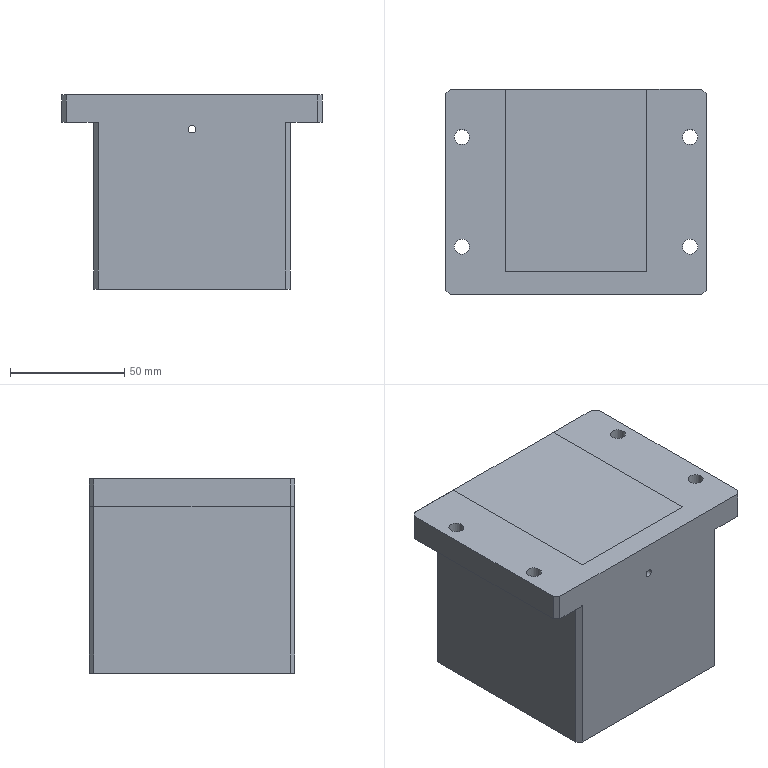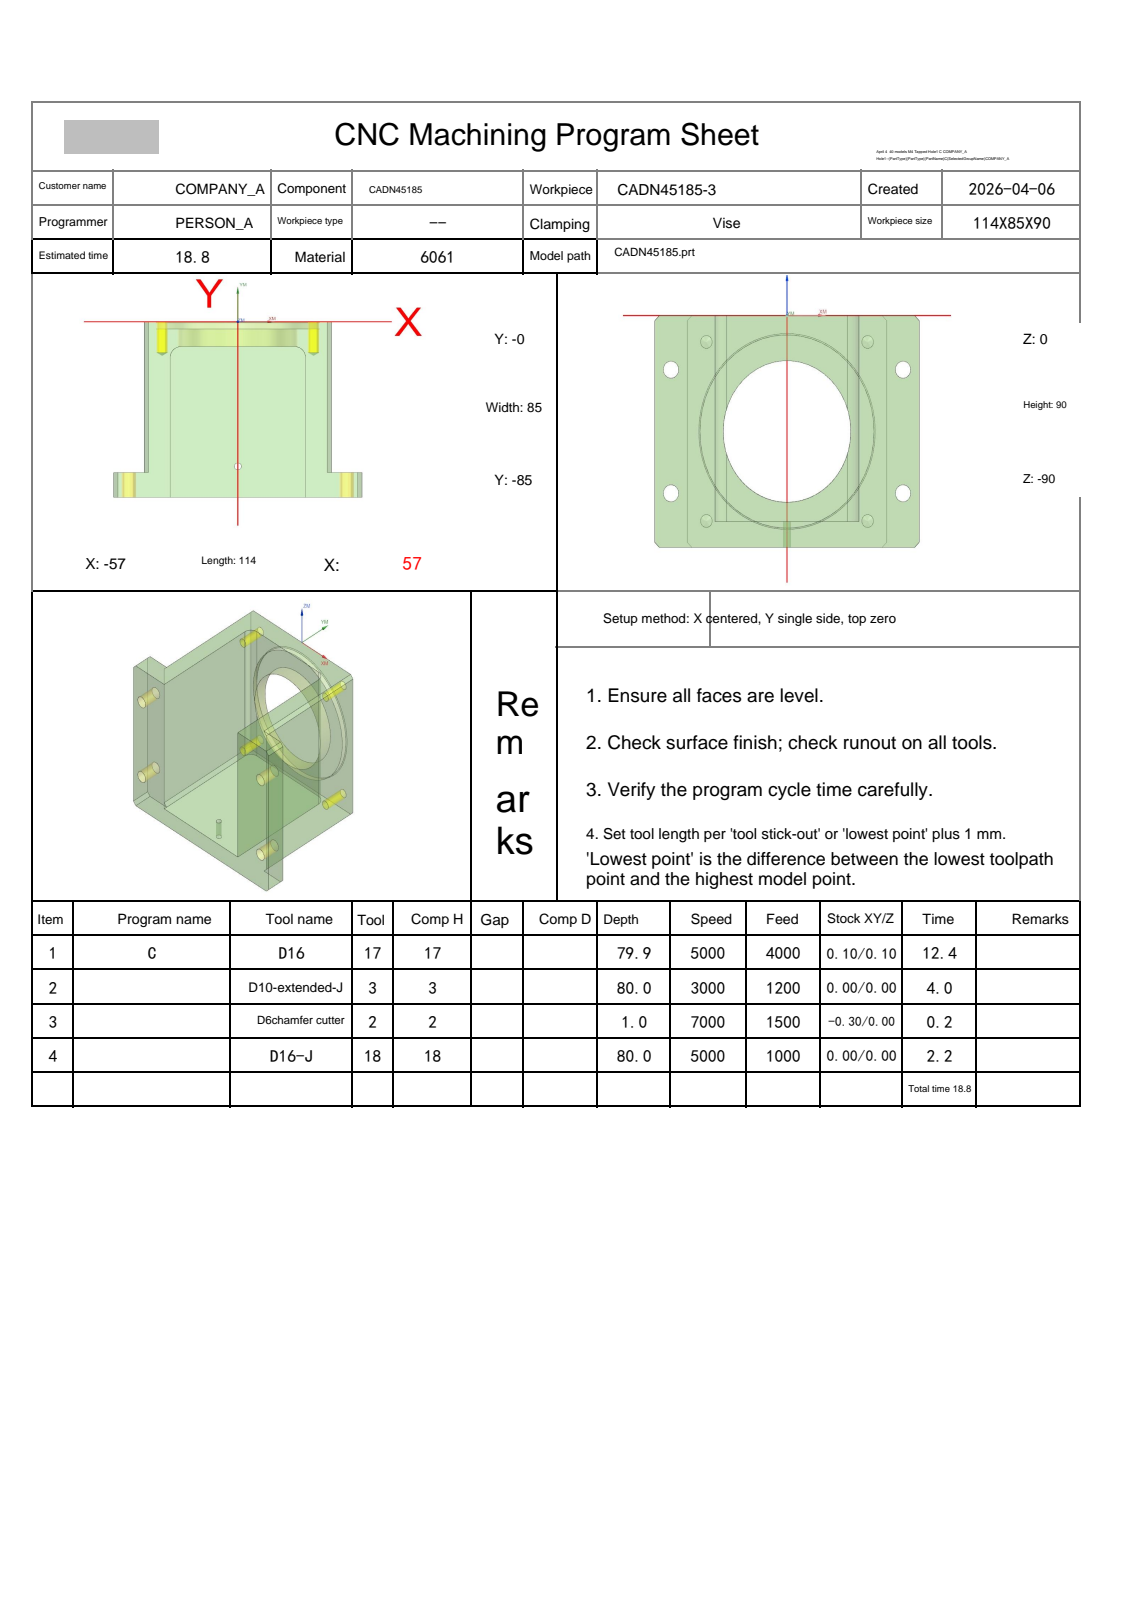NC program | NX | posted by the shop | part box 114 x 90 x 85 mm
Lines 2624 to 3642 of 14367:
N2 T03 M06
(D10-extended-J  D=10. R=0. H=03 ce=0.00 di=0.00)
G00 G90 G54 X24.999 Y-21.95 M03 S3000
G43 H03 Z50.
M08
Z.5
G01 X25.012 Y-21.947 Z.348 F1200.
X25.048 Y-21.938 Z.211
X25.103 Y-21.922 Z.089
X25.175 Y-21.899 Z-.02
X25.258 Y-21.868 Z-.115
X25.351 Y-21.828 Z-.198
X25.449 Y-21.778 Z-.269
X25.549 Y-21.718 Z-.329
X25.648 Y-21.647 Z-.378
X25.74 Y-21.564 Z-.419
X25.824 Y-21.469 Z-.45
X25.896 Y-21.361 Z-.473
X25.951 Y-21.238 Z-.488
X25.987 Y-21.102 Z-.497
X26. Y-20.95 Z-.5
Y-17.
X22.05
X21.955 Y-17.015 Z-.501
X21.88 Y-17.057 Z-.503
X21.826 Y-17.126 Z-.507
X21.791 Y-17.216 Z-.512
X21.774 Y-17.328 Z-.518
X21.775 Y-17.456 Z-.525
X21.79 Y-17.6 Z-.534
X21.821 Y-17.757 Z-.543
X21.864 Y-17.924 Z-.554
X21.92 Y-18.098 Z-.566
X21.987 Y-18.278 Z-.578
X22.064 Y-18.46 Z-.591
X22.15 Y-18.641 Z-.605
X22.243 Y-18.821 Z-.62
X22.485 Y-19.219 Z-.656
X22.761 Y-19.589 Z-.695
X23.07 Y-19.929 Z-.735
X23.41 Y-20.237 Z-.775
X23.78 Y-20.513 Z-.816
X24.179 Y-20.755 Z-.856
X24.358 Y-20.849 Z-.872
X24.54 Y-20.934 Z-.888
X24.722 Y-21.011 Z-.904
X24.901 Y-21.078 Z-.918
X25.076 Y-21.135 Z-.932
X25.243 Y-21.178 Z-.945
X25.399 Y-21.209 Z-.957
X25.543 Y-21.225 Z-.968
X25.672 Z-.977
X25.784 Y-21.209 Z-.985
X25.874 Y-21.174 Z-.991
X25.942 Y-21.12 Z-.996
X25.985 Y-21.045 Z-.999
X26. Y-20.95 Z-1.
Y-17.
X22.051
X21.955 Y-17.015 Z-1.001
X21.88 Y-17.057 Z-1.003
X21.826 Y-17.126 Z-1.007
X21.791 Y-17.216 Z-1.012
X21.774 Y-17.328 Z-1.018
Y-17.456 Z-1.025
X21.79 Y-17.6 Z-1.034
X21.82 Y-17.757 Z-1.044
X21.863 Y-17.924 Z-1.054
X21.919 Y-18.098 Z-1.066
X21.986 Y-18.278 Z-1.078
X22.063 Y-18.46 Z-1.091
X22.148 Y-18.641 Z-1.105
X22.241 Y-18.821 Z-1.12
X22.483 Y-19.219 Z-1.156
X22.759 Y-19.589 Z-1.195
X23.068 Y-19.929 Z-1.235
X23.408 Y-20.237 Z-1.276
X23.778 Y-20.513 Z-1.316
X24.178 Y-20.755 Z-1.356
X24.357 Y-20.849 Z-1.372
X24.539 Y-20.934 Z-1.388
X24.721 Y-21.011 Z-1.404
X24.901 Y-21.078 Z-1.418
X25.075 Y-21.135 Z-1.432
X25.242 Y-21.178 Z-1.445
X25.399 Y-21.209 Z-1.457
X25.543 Y-21.225 Z-1.468
X25.672 Z-1.477
X25.783 Y-21.209 Z-1.485
X25.874 Y-21.174 Z-1.491
X25.942 Y-21.12 Z-1.496
X25.985 Y-21.045 Z-1.499
X26. Y-20.95 Z-1.5
Y-17.
X22.051
X21.954 Y-17.015 Z-1.501
X21.88 Y-17.057 Z-1.503
X21.826 Y-17.126 Z-1.507
X21.791 Y-17.216 Z-1.512
X21.774 Y-17.328 Z-1.518
X21.773 Y-17.456 Z-1.525
X21.789 Y-17.6 Z-1.534
X21.819 Y-17.757 Z-1.544
X21.862 Y-17.924 Z-1.554
X21.918 Y-18.098 Z-1.566
X21.985 Y-18.278 Z-1.578
X22.061 Y-18.46 Z-1.592
X22.146 Y-18.641 Z-1.606
X22.239 Y-18.821 Z-1.62
X22.482 Y-19.22 Z-1.656
X22.758 Y-19.589 Z-1.695
X23.066 Y-19.929 Z-1.735
X23.406 Y-20.237 Z-1.776
X23.777 Y-20.513 Z-1.816
X24.177 Y-20.755 Z-1.856
X24.356 Y-20.849 Z-1.872
X24.538 Y-20.934 Z-1.888
X24.721 Y-21.011 Z-1.904
X24.9 Y-21.078 Z-1.918
X25.075 Y-21.135 Z-1.932
X25.242 Y-21.178 Z-1.945
X25.399 Y-21.209 Z-1.957
X25.543 Y-21.225 Z-1.968
X25.672 Z-1.977
X25.783 Y-21.209 Z-1.985
X25.874 Y-21.174 Z-1.991
X25.942 Y-21.12 Z-1.996
X25.985 Y-21.045 Z-1.999
X26. Y-20.95 Z-2.
Y-17.
X22.05
X21.954 Y-17.015 Z-2.001
X21.88 Y-17.057 Z-2.003
X21.826 Y-17.126 Z-2.007
X21.79 Y-17.216 Z-2.012
X21.773 Y-17.328 Z-2.018
Y-17.456 Z-2.025
X21.788 Y-17.601 Z-2.034
X21.818 Y-17.757 Z-2.044
X21.861 Y-17.924 Z-2.054
X21.917 Y-18.098 Z-2.066
X21.983 Y-18.278 Z-2.079
X22.059 Y-18.46 Z-2.092
X22.145 Y-18.641 Z-2.106
X22.238 Y-18.821 Z-2.12
X22.48 Y-19.22 Z-2.157
X22.756 Y-19.589 Z-2.195
X23.064 Y-19.929 Z-2.235
X23.405 Y-20.237 Z-2.276
X23.776 Y-20.513 Z-2.317
X24.176 Y-20.755 Z-2.356
X24.355 Y-20.849 Z-2.373
X24.538 Y-20.934 Z-2.388
X24.72 Y-21.011 Z-2.404
X24.9 Y-21.078 Z-2.419
X25.074 Y-21.135 Z-2.432
X25.241 Y-21.178 Z-2.445
X25.398 Y-21.209 Z-2.457
X25.543 Y-21.225 Z-2.468
X25.672 Z-2.477
X25.783 Y-21.209 Z-2.485
X25.874 Y-21.174 Z-2.491
X25.942 Y-21.12 Z-2.496
X25.985 Y-21.045 Z-2.499
X26. Y-20.95 Z-2.5
Y-17.
X22.05
X21.954 Y-17.015 Z-2.501
X21.88 Y-17.057 Z-2.503
X21.825 Y-17.126 Z-2.507
X21.79 Y-17.216 Z-2.512
X21.773 Y-17.328 Z-2.518
X21.772 Y-17.456 Z-2.526
X21.787 Y-17.601 Z-2.534
X21.817 Y-17.757 Z-2.544
X21.86 Y-17.924 Z-2.555
X21.915 Y-18.098 Z-2.566
X21.982 Y-18.278 Z-2.579
X22.058 Y-18.46 Z-2.592
X22.143 Y-18.641 Z-2.606
X22.236 Y-18.821 Z-2.621
X22.478 Y-19.22 Z-2.657
X22.754 Y-19.589 Z-2.695
X23.063 Y-19.929 Z-2.736
X23.403 Y-20.237 Z-2.776
X23.774 Y-20.513 Z-2.817
X24.175 Y-20.755 Z-2.856
X24.354 Y-20.849 Z-2.873
X24.537 Y-20.934 Z-2.889
X24.719 Y-21.011 Z-2.904
X24.899 Y-21.078 Z-2.919
X25.074 Y-21.135 Z-2.932
X25.241 Y-21.178 Z-2.945
X25.398 Y-21.209 Z-2.957
X25.543 Y-21.225 Z-2.968
X25.672 Z-2.977
X25.783 Y-21.209 Z-2.985
X25.874 Y-21.174 Z-2.991
X25.942 Y-21.12 Z-2.996
X25.985 Y-21.045 Z-2.999
X26. Y-20.95 Z-3.
Y-17.
X22.051
X21.954 Y-17.015 Z-3.001
X21.88 Y-17.057 Z-3.003
X21.825 Y-17.126 Z-3.007
X21.79 Y-17.216 Z-3.012
X21.772 Y-17.328 Z-3.018
Y-17.456 Z-3.026
X21.787 Y-17.601 Z-3.034
X21.816 Y-17.757 Z-3.044
X21.859 Y-17.924 Z-3.055
X21.914 Y-18.098 Z-3.066
X21.98 Y-18.278 Z-3.079
X22.056 Y-18.46 Z-3.092
X22.141 Y-18.642 Z-3.106
X22.234 Y-18.821 Z-3.121
X22.476 Y-19.22 Z-3.157
X22.752 Y-19.589 Z-3.196
X23.061 Y-19.929 Z-3.236
X23.402 Y-20.237 Z-3.276
X23.773 Y-20.513 Z-3.317
X24.174 Y-20.755 Z-3.356
X24.353 Y-20.849 Z-3.373
X24.536 Y-20.934 Z-3.389
X24.718 Y-21.011 Z-3.404
X24.898 Y-21.078 Z-3.419
X25.073 Y-21.135 Z-3.432
X25.241 Y-21.178 Z-3.445
X25.398 Y-21.209 Z-3.457
X25.542 Y-21.225 Z-3.468
X25.672 Z-3.477
X25.783 Y-21.209 Z-3.485
X25.874 Y-21.174 Z-3.491
X25.942 Y-21.12 Z-3.496
X25.985 Y-21.045 Z-3.499
X26. Y-20.95 Z-3.5
Y-17.
X22.05
X21.954 Y-17.015 Z-3.501
X21.88 Y-17.058 Z-3.503
X21.825 Y-17.126 Z-3.507
X21.789 Y-17.216 Z-3.512
X21.772 Y-17.328 Z-3.518
X21.771 Y-17.456 Z-3.526
X21.786 Y-17.601 Z-3.534
X21.815 Y-17.757 Z-3.544
X21.858 Y-17.924 Z-3.555
X21.913 Y-18.098 Z-3.567
X21.979 Y-18.278 Z-3.579
X22.055 Y-18.46 Z-3.592
X22.139 Y-18.642 Z-3.606
X22.232 Y-18.821 Z-3.621
X22.474 Y-19.22 Z-3.657
X22.75 Y-19.589 Z-3.696
X23.059 Y-19.929 Z-3.736
X23.4 Y-20.237 Z-3.777
X23.772 Y-20.513 Z-3.817
X24.173 Y-20.755 Z-3.856
X24.353 Y-20.849 Z-3.873
X24.535 Y-20.934 Z-3.889
X24.718 Y-21.011 Z-3.904
X24.898 Y-21.078 Z-3.919
X25.073 Y-21.135 Z-3.933
X25.24 Y-21.178 Z-3.945
X25.398 Y-21.209 Z-3.957
X25.542 Y-21.225 Z-3.968
X25.671 Z-3.977
X25.783 Y-21.209 Z-3.985
X25.874 Y-21.174 Z-3.991
X25.942 Y-21.12 Z-3.996
X25.985 Y-21.045 Z-3.999
X26. Y-20.95 Z-4.
Y-17.
X22.05
X21.954 Y-17.015 Z-4.001
X21.88 Y-17.058 Z-4.003
X21.825 Y-17.126 Z-4.007
X21.789 Y-17.216 Z-4.012
X21.771 Y-17.328 Z-4.018
X21.77 Y-17.456 Z-4.026
X21.785 Y-17.601 Z-4.034
X21.814 Y-17.757 Z-4.044
X21.857 Y-17.924 Z-4.055
X21.911 Y-18.098 Z-4.067
X21.977 Y-18.278 Z-4.079
X22.053 Y-18.46 Z-4.093
X22.138 Y-18.642 Z-4.107
X22.23 Y-18.821 Z-4.121
X22.472 Y-19.22 Z-4.158
X22.748 Y-19.589 Z-4.196
X23.057 Y-19.929 Z-4.236
X23.399 Y-20.237 Z-4.277
X23.77 Y-20.513 Z-4.317
X24.172 Y-20.755 Z-4.357
X24.352 Y-20.849 Z-4.373
X24.534 Y-20.934 Z-4.389
X24.717 Y-21.011 Z-4.404
X24.897 Y-21.078 Z-4.419
X25.072 Y-21.135 Z-4.433
X25.24 Y-21.178 Z-4.445
X25.397 Y-21.209 Z-4.457
X25.542 Y-21.225 Z-4.468
X25.671 Z-4.477
X25.783 Y-21.209 Z-4.485
X25.874 Y-21.174 Z-4.491
X25.942 Y-21.12 Z-4.496
X25.985 Y-21.045 Z-4.499
X26. Y-20.95 Z-4.5
Y-17.
X22.051
X21.954 Y-17.015 Z-4.501
X21.879 Y-17.058 Z-4.503
X21.825 Y-17.126 Z-4.507
X21.789 Y-17.216 Z-4.512
X21.771 Y-17.328 Z-4.518
X21.77 Y-17.456 Z-4.526
X21.784 Y-17.601 Z-4.535
X21.813 Y-17.757 Z-4.544
X21.855 Y-17.924 Z-4.555
X21.91 Y-18.099 Z-4.567
X21.976 Y-18.278 Z-4.579
X22.051 Y-18.46 Z-4.593
X22.136 Y-18.642 Z-4.607
X22.228 Y-18.821 Z-4.621
X22.47 Y-19.22 Z-4.658
X22.746 Y-19.589 Z-4.696
X23.055 Y-19.929 Z-4.736
X23.397 Y-20.237 Z-4.777
X23.769 Y-20.513 Z-4.817
X24.17 Y-20.756 Z-4.857
X24.351 Y-20.849 Z-4.873
X24.534 Y-20.934 Z-4.889
X24.716 Y-21.011 Z-4.904
X24.897 Y-21.078 Z-4.919
X25.072 Y-21.135 Z-4.933
X25.239 Y-21.178 Z-4.945
X25.397 Y-21.209 Z-4.957
X25.542 Y-21.225 Z-4.968
X25.671 Z-4.977
X25.783 Y-21.209 Z-4.985
X25.874 Y-21.174 Z-4.991
X25.942 Y-21.12 Z-4.996
X25.985 Y-21.045 Z-4.999
X26. Y-20.95 Z-5.
Y-17.
X22.05
X21.954 Y-17.015 Z-5.001
X21.879 Y-17.058 Z-5.003
X21.824 Y-17.126 Z-5.007
X21.789 Y-17.216 Z-5.012
X21.771 Y-17.328 Z-5.018
X21.769 Y-17.457 Z-5.026
X21.783 Y-17.601 Z-5.035
X21.812 Y-17.757 Z-5.044
X21.854 Y-17.924 Z-5.055
X21.909 Y-18.099 Z-5.067
X21.974 Y-18.278 Z-5.08
X22.05 Y-18.46 Z-5.093
X22.134 Y-18.642 Z-5.107
X22.227 Y-18.821 Z-5.122
X22.468 Y-19.22 Z-5.158
X22.744 Y-19.59 Z-5.197
X23.054 Y-19.929 Z-5.237
X23.395 Y-20.237 Z-5.277
X23.768 Y-20.513 Z-5.317
X24.169 Y-20.756 Z-5.357
X24.35 Y-20.849 Z-5.373
X24.533 Y-20.934 Z-5.389
X24.716 Y-21.011 Z-5.404
X24.896 Y-21.079 Z-5.419
X25.071 Y-21.135 Z-5.433
X25.239 Y-21.178 Z-5.446
X25.397 Y-21.209 Z-5.457
X25.541 Y-21.225 Z-5.468
X25.671 Z-5.477
X25.783 Y-21.209 Z-5.485
X25.874 Y-21.174 Z-5.491
X25.942 Y-21.12 Z-5.496
X25.985 Y-21.045 Z-5.499
X26. Y-20.95 Z-5.5
Y-17.
X22.05
X21.954 Y-17.015 Z-5.501
X21.879 Y-17.058 Z-5.503
X21.824 Y-17.126 Z-5.507
X21.788 Y-17.216 Z-5.512
X21.77 Y-17.328 Z-5.518
X21.769 Y-17.457 Z-5.526
X21.783 Y-17.601 Z-5.535
X21.811 Y-17.757 Z-5.545
X21.853 Y-17.924 Z-5.555
X21.907 Y-18.099 Z-5.567
X21.973 Y-18.278 Z-5.58
X22.048 Y-18.46 Z-5.593
X22.133 Y-18.642 Z-5.607
X22.225 Y-18.821 Z-5.622
X22.466 Y-19.22 Z-5.658
X22.742 Y-19.59 Z-5.697
X23.052 Y-19.929 Z-5.737
X23.394 Y-20.237 Z-5.777
X23.766 Y-20.513 Z-5.818
X24.168 Y-20.756 Z-5.857
X24.349 Y-20.849 Z-5.873
X24.532 Y-20.934 Z-5.889
X24.715 Y-21.011 Z-5.904
X24.895 Y-21.079 Z-5.919
X25.071 Y-21.135 Z-5.933
X25.239 Y-21.178 Z-5.946
X25.396 Y-21.209 Z-5.957
X25.541 Y-21.225 Z-5.968
X25.671 Z-5.977
X25.782 Y-21.209 Z-5.985
X25.874 Y-21.174 Z-5.991
X25.942 Y-21.12 Z-5.996
X25.985 Y-21.045 Z-5.999
X26. Y-20.95 Z-6.
Y-17.
X22.051
X21.954 Y-17.015 Z-6.001
X21.879 Y-17.058 Z-6.003
X21.824 Y-17.126 Z-6.007
X21.788 Y-17.216 Z-6.012
X21.77 Y-17.328 Z-6.018
X21.768 Y-17.457 Z-6.026
X21.782 Y-17.601 Z-6.035
X21.81 Y-17.757 Z-6.045
X21.852 Y-17.924 Z-6.056
X21.906 Y-18.099 Z-6.067
X21.971 Y-18.278 Z-6.08
X22.047 Y-18.46 Z-6.093
X22.131 Y-18.642 Z-6.107
X22.223 Y-18.821 Z-6.122
X22.464 Y-19.22 Z-6.158
X22.74 Y-19.59 Z-6.197
X23.05 Y-19.929 Z-6.237
X23.392 Y-20.237 Z-6.277
X23.765 Y-20.513 Z-6.318
X24.167 Y-20.756 Z-6.357
X24.348 Y-20.849 Z-6.373
X24.531 Y-20.934 Z-6.389
X24.714 Y-21.011 Z-6.404
X24.895 Y-21.079 Z-6.419
X25.07 Y-21.135 Z-6.433
X25.238 Y-21.178 Z-6.446
X25.396 Y-21.209 Z-6.457
X25.541 Y-21.225 Z-6.468
X25.671 Z-6.477
X25.782 Y-21.209 Z-6.485
X25.874 Y-21.174 Z-6.491
X25.942 Y-21.12 Z-6.496
X25.985 Y-21.045 Z-6.499
X26. Y-20.95 Z-6.5
Y-17.
X22.05
X21.954 Y-17.015 Z-6.501
X21.879 Y-17.058 Z-6.503
X21.824 Y-17.126 Z-6.507
X21.788 Y-17.216 Z-6.512
X21.769 Y-17.328 Z-6.518
X21.767 Y-17.457 Z-6.526
X21.781 Y-17.601 Z-6.535
X21.809 Y-17.757 Z-6.545
X21.851 Y-17.924 Z-6.556
X21.905 Y-18.099 Z-6.567
X21.97 Y-18.278 Z-6.58
X22.045 Y-18.46 Z-6.593
X22.129 Y-18.642 Z-6.608
X22.221 Y-18.821 Z-6.622
X22.462 Y-19.22 Z-6.659
X22.738 Y-19.59 Z-6.697
X23.048 Y-19.929 Z-6.737
X23.391 Y-20.237 Z-6.778
X23.764 Y-20.513 Z-6.818
X24.166 Y-20.756 Z-6.857
X24.347 Y-20.849 Z-6.873
X24.53 Y-20.934 Z-6.889
X24.714 Y-21.011 Z-6.905
X24.894 Y-21.079 Z-6.919
X25.07 Y-21.135 Z-6.933
X25.238 Y-21.179 Z-6.946
X25.396 Y-21.209 Z-6.957
X25.541 Y-21.225 Z-6.968
X25.67 Z-6.977
X25.782 Y-21.209 Z-6.985
X25.874 Y-21.174 Z-6.991
X25.942 Y-21.12 Z-6.996
X25.985 Y-21.045 Z-6.999
X26. Y-20.95 Z-7.
Y-17.
X22.051
X21.954 Y-17.015 Z-7.001
X21.879 Y-17.058 Z-7.003
X21.824 Y-17.126 Z-7.007
X21.787 Y-17.216 Z-7.012
X21.769 Y-17.328 Z-7.018
X21.767 Y-17.457 Z-7.026
X21.78 Y-17.601 Z-7.035
X21.808 Y-17.757 Z-7.045
X21.85 Y-17.924 Z-7.056
X21.904 Y-18.099 Z-7.068
X21.968 Y-18.278 Z-7.08
X22.043 Y-18.46 Z-7.094
X22.127 Y-18.642 Z-7.108
X22.219 Y-18.821 Z-7.123
X22.46 Y-19.22 Z-7.159
X22.736 Y-19.59 Z-7.197
X23.046 Y-19.929 Z-7.237
X23.389 Y-20.237 Z-7.278
X23.763 Y-20.513 Z-7.318
X24.165 Y-20.756 Z-7.357
X24.346 Y-20.849 Z-7.374
X24.529 Y-20.934 Z-7.389
X24.713 Y-21.011 Z-7.405
X24.894 Y-21.079 Z-7.419
X25.069 Y-21.135 Z-7.433
X25.238 Y-21.179 Z-7.446
X25.395 Y-21.209 Z-7.457
X25.54 Y-21.225 Z-7.468
X25.67 Z-7.477
X25.782 Y-21.209 Z-7.485
X25.874 Y-21.174 Z-7.491
X25.942 Y-21.12 Z-7.496
X25.985 Y-21.045 Z-7.499
X26. Y-20.95 Z-7.5
Y-17.
X22.051
X21.954 Y-17.015 Z-7.501
X21.879 Y-17.058 Z-7.503
X21.824 Y-17.126 Z-7.507
X21.787 Y-17.216 Z-7.512
X21.768 Y-17.328 Z-7.519
X21.766 Y-17.457 Z-7.526
X21.78 Y-17.601 Z-7.535
X21.807 Y-17.757 Z-7.545
X21.849 Y-17.924 Z-7.556
X21.902 Y-18.099 Z-7.568
X21.967 Y-18.278 Z-7.58
X22.042 Y-18.46 Z-7.594
X22.126 Y-18.642 Z-7.608
X22.217 Y-18.821 Z-7.623
X22.458 Y-19.22 Z-7.659
X22.734 Y-19.59 Z-7.698
X23.045 Y-19.929 Z-7.738
X23.387 Y-20.237 Z-7.778
X23.761 Y-20.513 Z-7.818
X24.164 Y-20.756 Z-7.857
X24.345 Y-20.849 Z-7.874
X24.529 Y-20.934 Z-7.889
X24.712 Y-21.011 Z-7.905
X24.893 Y-21.079 Z-7.919
X25.069 Y-21.135 Z-7.933
X25.237 Y-21.179 Z-7.946
X25.395 Y-21.209 Z-7.958
X25.54 Y-21.225 Z-7.968
X25.67 Z-7.977
X25.782 Y-21.209 Z-7.985
X25.874 Y-21.174 Z-7.991
X25.942 Y-21.12 Z-7.996
X25.985 Y-21.045 Z-7.999
X26. Y-20.95 Z-8.
Y-17.
X22.05
X21.954 Y-17.015 Z-8.001
X21.879 Y-17.058 Z-8.003
X21.823 Y-17.126 Z-8.007
X21.787 Y-17.216 Z-8.012
X21.768 Y-17.328 Z-8.019
X21.766 Y-17.457 Z-8.026
X21.779 Y-17.601 Z-8.035
X21.807 Y-17.757 Z-8.045
X21.848 Y-17.924 Z-8.056
X21.901 Y-18.099 Z-8.068
X21.965 Y-18.278 Z-8.081
X22.04 Y-18.46 Z-8.094
X22.124 Y-18.642 Z-8.108
X22.215 Y-18.821 Z-8.123
X22.456 Y-19.22 Z-8.159
X22.732 Y-19.59 Z-8.198
X23.043 Y-19.929 Z-8.238
X23.386 Y-20.237 Z-8.278
X23.76 Y-20.513 Z-8.318
X24.163 Y-20.756 Z-8.358
X24.344 Y-20.849 Z-8.374
X24.528 Y-20.934 Z-8.39
X24.711 Y-21.011 Z-8.405
X24.893 Y-21.079 Z-8.419
X25.068 Y-21.135 Z-8.433
X25.237 Y-21.179 Z-8.446
X25.395 Y-21.209 Z-8.458
X25.54 Y-21.225 Z-8.468
X25.67 Z-8.477
X25.782 Y-21.209 Z-8.485
X25.874 Y-21.174 Z-8.491
X25.942 Y-21.12 Z-8.496
X25.985 Y-21.045 Z-8.499
X26. Y-20.95 Z-8.5
Y-17.
X22.05
X21.954 Y-17.015 Z-8.501
X21.879 Y-17.058 Z-8.503
X21.823 Y-17.126 Z-8.507
X21.787 Y-17.216 Z-8.512
X21.767 Y-17.328 Z-8.519
X21.765 Y-17.457 Z-8.526
X21.778 Y-17.601 Z-8.535
X21.806 Y-17.757 Z-8.545
X21.846 Y-17.924 Z-8.556
X21.9 Y-18.099 Z-8.568
X21.964 Y-18.278 Z-8.581
X22.039 Y-18.46 Z-8.594
X22.122 Y-18.642 Z-8.608
X22.214 Y-18.821 Z-8.623
X22.454 Y-19.22 Z-8.66
X22.73 Y-19.59 Z-8.698
X23.041 Y-19.929 Z-8.738
X23.384 Y-20.237 Z-8.778
X23.759 Y-20.513 Z-8.819
X24.162 Y-20.756 Z-8.858
X24.343 Y-20.849 Z-8.874
X24.527 Y-20.934 Z-8.89
X24.711 Y-21.011 Z-8.905
X24.892 Y-21.079 Z-8.919
X25.068 Y-21.135 Z-8.933
X25.236 Y-21.179 Z-8.946
X25.394 Y-21.209 Z-8.958
X25.54 Y-21.225 Z-8.968
X25.67 Z-8.977
X25.782 Y-21.209 Z-8.985
X25.873 Y-21.174 Z-8.991
X25.942 Y-21.12 Z-8.996
X25.985 Y-21.045 Z-8.999
X26. Y-20.95 Z-9.
Y-17.
X22.051
X21.954 Y-17.015 Z-9.001
X21.879 Y-17.058 Z-9.003
X21.823 Y-17.126 Z-9.007
X21.786 Y-17.216 Z-9.012
X21.767 Y-17.328 Z-9.019
X21.764 Y-17.457 Z-9.026
X21.777 Y-17.601 Z-9.035
X21.805 Y-17.757 Z-9.045
X21.845 Y-17.924 Z-9.056
X21.898 Y-18.099 Z-9.068
X21.963 Y-18.278 Z-9.081
X22.037 Y-18.46 Z-9.094
X22.12 Y-18.642 Z-9.109
X22.212 Y-18.821 Z-9.123
X22.416 Y-19.165 Z-9.154
X22.646 Y-19.487 Z-9.187
X22.902 Y-19.787 Z-9.221
X23.183 Y-20.065 Z-9.256
X23.487 Y-20.32 Z-9.29
X23.813 Y-20.55 Z-9.324
X24.161 Y-20.756 Z-9.358
X24.342 Y-20.849 Z-9.374
X24.526 Y-20.934 Z-9.39
X24.71 Y-21.011 Z-9.405
X24.891 Y-21.079 Z-9.419
X25.067 Y-21.135 Z-9.433
X25.236 Y-21.179 Z-9.446
X25.394 Y-21.209 Z-9.458
X25.54 Y-21.225 Z-9.468
X25.67 Z-9.477
X25.782 Y-21.209 Z-9.485
X25.873 Y-21.174 Z-9.491
X25.942 Y-21.12 Z-9.496
X25.985 Y-21.045 Z-9.499
X26. Y-20.95 Z-9.5
Y-17.
X22.05
X21.954 Y-17.015 Z-9.501
X21.879 Y-17.058 Z-9.503
X21.823 Y-17.126 Z-9.507
X21.786 Y-17.216 Z-9.512
X21.767 Y-17.328 Z-9.519
X21.764 Y-17.457 Z-9.527
X21.777 Y-17.601 Z-9.535
X21.804 Y-17.757 Z-9.545
X21.844 Y-17.924 Z-9.556
X21.897 Y-18.099 Z-9.568
X21.961 Y-18.278 Z-9.581
X22.035 Y-18.46 Z-9.595
X22.119 Y-18.642 Z-9.609
X22.21 Y-18.821 Z-9.624
X22.414 Y-19.165 Z-9.655
X22.644 Y-19.487 Z-9.687
X22.9 Y-19.787 Z-9.721
X23.181 Y-20.065 Z-9.756
X23.485 Y-20.32 Z-9.79
X23.812 Y-20.55 Z-9.825
X24.16 Y-20.756 Z-9.858
X24.342 Y-20.849 Z-9.874
X24.525 Y-20.934 Z-9.89
X24.709 Y-21.011 Z-9.905
X24.891 Y-21.079 Z-9.92
X25.067 Y-21.135 Z-9.933
X25.236 Y-21.179 Z-9.946
X25.394 Y-21.209 Z-9.958
X25.539 Y-21.225 Z-9.968
X25.669 Z-9.977
X25.782 Y-21.209 Z-9.985
X25.873 Y-21.174 Z-9.992
X25.942 Y-21.12 Z-9.996
X25.985 Y-21.045 Z-9.999
X26. Y-20.95 Z-10.
Y-17.
X22.051
X21.954 Y-17.015 Z-10.001
X21.879 Y-17.058 Z-10.003
X21.823 Y-17.126 Z-10.007
X21.786 Y-17.216 Z-10.012
X21.766 Y-17.328 Z-10.019
X21.763 Y-17.457 Z-10.027
X21.776 Y-17.601 Z-10.036
X21.803 Y-17.757 Z-10.046
X21.843 Y-17.924 Z-10.057
X21.896 Y-18.099 Z-10.068
X21.96 Y-18.278 Z-10.081
X22.034 Y-18.46 Z-10.095
X22.117 Y-18.642 Z-10.109
X22.208 Y-18.821 Z-10.124
X22.412 Y-19.165 Z-10.155
X22.642 Y-19.487 Z-10.188
X22.898 Y-19.787 Z-10.221
X23.179 Y-20.065 Z-10.256
X23.484 Y-20.32 Z-10.29
X23.811 Y-20.55 Z-10.325
X24.159 Y-20.756 Z-10.358
X24.341 Y-20.849 Z-10.374
X24.525 Y-20.934 Z-10.39
X24.709 Y-21.011 Z-10.405
X24.89 Y-21.079 Z-10.42
X25.066 Y-21.135 Z-10.433
X25.235 Y-21.179 Z-10.446
X25.394 Y-21.209 Z-10.458
X25.539 Y-21.225 Z-10.468
X25.669 Z-10.477
X25.781 Y-21.209 Z-10.485
X25.873 Y-21.174 Z-10.492
X25.942 Y-21.12 Z-10.496
X25.985 Y-21.045 Z-10.499
X26. Y-20.95 Z-10.5
Y-17.
X22.05
X21.954 Y-17.015 Z-10.501
X21.878 Y-17.058 Z-10.503
X21.823 Y-17.126 Z-10.507
X21.785 Y-17.216 Z-10.512
X21.766 Y-17.328 Z-10.519
X21.763 Y-17.457 Z-10.527
X21.775 Y-17.601 Z-10.536
X21.802 Y-17.757 Z-10.546
X21.842 Y-17.924 Z-10.557
X21.894 Y-18.099 Z-10.569
X21.958 Y-18.278 Z-10.581
X22.032 Y-18.46 Z-10.595
X22.115 Y-18.642 Z-10.609
X22.206 Y-18.821 Z-10.624
X22.41 Y-19.165 Z-10.655
X22.64 Y-19.487 Z-10.688
X22.896 Y-19.787 Z-10.722
X23.177 Y-20.065 Z-10.756
X23.482 Y-20.32 Z-10.791
X23.809 Y-20.55 Z-10.825
X24.158 Y-20.756 Z-10.858
X24.34 Y-20.849 Z-10.874
X24.524 Y-20.934 Z-10.89
X24.708 Y-21.011 Z-10.905
X24.89 Y-21.079 Z-10.92
X25.066 Y-21.135 Z-10.933
X25.235 Y-21.179 Z-10.946
X25.393 Y-21.209 Z-10.958
X25.539 Y-21.225 Z-10.968
X25.669 Z-10.977
X25.781 Y-21.209 Z-10.985
X25.873 Y-21.174 Z-10.992
X25.942 Y-21.12 Z-10.996
X25.985 Y-21.045 Z-10.999
X26. Y-20.95 Z-11.
Y-17.
X22.051
X21.954 Y-17.015 Z-11.001
X21.878 Y-17.058 Z-11.003
X21.822 Y-17.126 Z-11.007
X21.785 Y-17.216 Z-11.012
X21.765 Y-17.328 Z-11.019
X21.762 Y-17.457 Z-11.027
X21.774 Y-17.601 Z-11.036
X21.801 Y-17.757 Z-11.046
X21.841 Y-17.924 Z-11.057
X21.893 Y-18.099 Z-11.069
X21.957 Y-18.278 Z-11.082
X22.03 Y-18.46 Z-11.095
X22.113 Y-18.642 Z-11.109
X22.204 Y-18.821 Z-11.124
X22.408 Y-19.165 Z-11.155
X22.638 Y-19.487 Z-11.188
X22.894 Y-19.787 Z-11.222
X23.176 Y-20.065 Z-11.256
X23.481 Y-20.32 Z-11.291
X23.808 Y-20.55 Z-11.325
X24.157 Y-20.756 Z-11.358
X24.339 Y-20.849 Z-11.374
X24.523 Y-20.934 Z-11.39
X24.707 Y-21.011 Z-11.405
X24.889 Y-21.079 Z-11.42
X25.066 Y-21.135 Z-11.433
X25.234 Y-21.179 Z-11.446
X25.393 Y-21.209 Z-11.458
X25.539 Y-21.225 Z-11.468
X25.669 Z-11.477
X25.781 Y-21.209 Z-11.485
X25.873 Y-21.174 Z-11.492
X25.942 Y-21.12 Z-11.496
X25.985 Y-21.045 Z-11.499
X26. Y-20.95 Z-11.5
Y-17.
X22.051
X21.954 Y-17.015 Z-11.501
X21.878 Y-17.058 Z-11.503
X21.822 Y-17.126 Z-11.507
X21.785 Y-17.216 Z-11.512
X21.765 Y-17.328 Z-11.519
X21.761 Y-17.457 Z-11.527
X21.773 Y-17.601 Z-11.536
X21.8 Y-17.757 Z-11.546
X21.84 Y-17.924 Z-11.557
X21.892 Y-18.099 Z-11.569
X21.955 Y-18.278 Z-11.582
X22.029 Y-18.46 Z-11.595
X22.112 Y-18.642 Z-11.61
X22.203 Y-18.821 Z-11.624
X22.406 Y-19.165 Z-11.656
X22.636 Y-19.487 Z-11.688
X22.893 Y-19.787 Z-11.722
X23.174 Y-20.065 Z-11.757
X23.479 Y-20.32 Z-11.791
X23.807 Y-20.55 Z-11.825
X24.156 Y-20.756 Z-11.858
X24.338 Y-20.849 Z-11.875
X24.522 Y-20.934 Z-11.89
X24.707 Y-21.011 Z-11.905
X24.888 Y-21.079 Z-11.92
X25.065 Y-21.135 Z-11.933
X25.234 Y-21.179 Z-11.946
X25.393 Y-21.209 Z-11.958
X25.538 Y-21.225 Z-11.968
X25.669 Z-11.977
X25.781 Y-21.209 Z-11.985
X25.873 Y-21.174 Z-11.992
X25.942 Y-21.12 Z-11.996
X25.985 Y-21.045 Z-11.999
X26. Y-20.95 Z-12.
Y-17.
X22.05
X21.954 Y-17.015 Z-12.001
X21.878 Y-17.058 Z-12.003
X21.822 Y-17.126 Z-12.007
X21.784 Y-17.216 Z-12.012
X21.764 Y-17.328 Z-12.019
X21.761 Y-17.457 Z-12.027
X21.773 Y-17.601 Z-12.036
X21.799 Y-17.757 Z-12.046
X21.839 Y-17.924 Z-12.057
X21.891 Y-18.099 Z-12.069
X21.954 Y-18.278 Z-12.082
X22.027 Y-18.46 Z-12.096
X22.11 Y-18.642 Z-12.11
X22.201 Y-18.821 Z-12.125
X22.404 Y-19.165 Z-12.156
X22.634 Y-19.487 Z-12.189
X22.891 Y-19.787 Z-12.222
X23.172 Y-20.065 Z-12.257
X23.478 Y-20.32 Z-12.291
X23.805 Y-20.55 Z-12.325
X24.155 Y-20.756 Z-12.359
X24.337 Y-20.849 Z-12.375
X24.521 Y-20.934 Z-12.39
X24.706 Y-21.011 Z-12.405
X24.888 Y-21.079 Z-12.42
X25.065 Y-21.135 Z-12.434
X25.234 Y-21.179 Z-12.446
X25.392 Y-21.209 Z-12.458
X25.538 Y-21.225 Z-12.468
X25.669 Z-12.477
X25.781 Y-21.209 Z-12.485
X25.873 Y-21.174 Z-12.492
X25.942 Y-21.12 Z-12.496
X25.985 Y-21.045 Z-12.499
X26. Y-20.95 Z-12.5
Y-17.
X22.05
X21.954 Y-17.015 Z-12.501
X21.878 Y-17.058 Z-12.503
X21.822 Y-17.126 Z-12.507
X21.784 Y-17.216 Z-12.512
X21.764 Y-17.328 Z-12.519
X21.76 Y-17.457 Z-12.527
X21.772 Y-17.601 Z-12.536
X21.798 Y-17.757 Z-12.546
X21.837 Y-17.924 Z-12.557
X21.889 Y-18.099 Z-12.569
X21.952 Y-18.278 Z-12.582
X22.026 Y-18.46 Z-12.596
X22.108 Y-18.642 Z-12.61
X22.199 Y-18.821 Z-12.625
X22.402 Y-19.165 Z-12.656
X22.632 Y-19.487 Z-12.689
X22.889 Y-19.787 Z-12.723
X23.171 Y-20.065 Z-12.757
X23.476 Y-20.319 Z-12.791
X23.804 Y-20.55 Z-12.825
X24.154 Y-20.756 Z-12.859
X24.336 Y-20.849 Z-12.875
X24.521 Y-20.934 Z-12.89
X24.705 Y-21.011 Z-12.906
X24.887 Y-21.079 Z-12.92
X25.064 Y-21.135 Z-12.934
X25.233 Y-21.178 Z-12.946
X25.392 Y-21.209 Z-12.958
X25.538 Y-21.225 Z-12.968
X25.668 Z-12.978
X25.781 Y-21.209 Z-12.985
X25.873 Y-21.174 Z-12.992
X25.942 Y-21.12 Z-12.996
X25.985 Y-21.045 Z-12.999
X26. Y-20.95 Z-13.
Y-17.
X22.051
X21.954 Y-17.015 Z-13.001
X21.878 Y-17.058 Z-13.003
X21.822 Y-17.126 Z-13.007
X21.784 Y-17.216 Z-13.012
X21.763 Y-17.328 Z-13.019
X21.76 Y-17.457 Z-13.027
X21.771 Y-17.601 Z-13.036
X21.797 Y-17.757 Z-13.046
X21.836 Y-17.924 Z-13.057
X21.888 Y-18.099 Z-13.069
X21.951 Y-18.278 Z-13.082
X22.024 Y-18.46 Z-13.096
X22.106 Y-18.642 Z-13.11
X22.197 Y-18.821 Z-13.125
X22.4 Y-19.165 Z-13.156
X22.63 Y-19.487 Z-13.189
X22.887 Y-19.787 Z-13.223
X23.169 Y-20.065 Z-13.257
X23.474 Y-20.319 Z-13.292
X23.803 Y-20.55 Z-13.326
X24.153 Y-20.756 Z-13.359
X24.335 Y-20.849 Z-13.375
X24.52 Y-20.934 Z-13.391
X24.705 Y-21.011 Z-13.406
X24.887 Y-21.079 Z-13.42
X25.064 Y-21.135 Z-13.434
X25.233 Y-21.178 Z-13.446
X25.392 Y-21.209 Z-13.458
X25.538 Y-21.225 Z-13.468
X25.668 Z-13.478
X25.781 Y-21.209 Z-13.485
X25.873 Y-21.174 Z-13.492
X25.942 Y-21.12 Z-13.496
X25.985 Y-21.045 Z-13.499
X26. Y-20.95 Z-13.5
Y-17.
X22.05
X21.954 Y-17.015 Z-13.501
X21.878 Y-17.058 Z-13.503
X21.822 Y-17.126 Z-13.507
X21.784 Y-17.216 Z-13.512
X21.763 Y-17.328 Z-13.519
X21.759 Y-17.456 Z-13.527
X21.77 Y-17.601 Z-13.536
X21.796 Y-17.757 Z-13.546
X21.835 Y-17.924 Z-13.557
X21.887 Y-18.099 Z-13.57
X21.949 Y-18.278 Z-13.582
X22.022 Y-18.46 Z-13.596
X22.105 Y-18.642 Z-13.61
X22.195 Y-18.821 Z-13.625
X22.398 Y-19.164 Z-13.657
X22.628 Y-19.487 Z-13.689
X22.885 Y-19.787 Z-13.723
X23.167 Y-20.065 Z-13.757
X23.473 Y-20.319 Z-13.792
X23.802 Y-20.55 Z-13.826
X24.152 Y-20.756 Z-13.859
X24.334 Y-20.849 Z-13.875
X24.519 Y-20.934 Z-13.891
X24.704 Y-21.011 Z-13.906
X24.886 Y-21.078 Z-13.92
X25.063 Y-21.135 Z-13.934
X25.232 Y-21.178 Z-13.946
X25.391 Y-21.209 Z-13.958
X25.537 Y-21.225 Z-13.968
X25.668 Z-13.978
X25.781 Y-21.209 Z-13.985
X25.873 Y-21.174 Z-13.992
X25.942 Y-21.12 Z-13.996
X25.985 Y-21.045 Z-13.999
X26. Y-20.95 Z-14.
Y-17.
X22.051
X21.954 Y-17.015 Z-14.001
X21.878 Y-17.058 Z-14.003
X21.821 Y-17.126 Z-14.007
X21.783 Y-17.216 Z-14.013
X21.763 Y-17.328 Z-14.019
X21.758 Y-17.456 Z-14.027
X21.77 Y-17.601 Z-14.036
X21.795 Y-17.757 Z-14.046
X21.834 Y-17.924 Z-14.058
X21.885 Y-18.098 Z-14.07
X21.948 Y-18.278 Z-14.083
X22.021 Y-18.46 Z-14.096
X22.103 Y-18.642 Z-14.111
X22.193 Y-18.821 Z-14.126